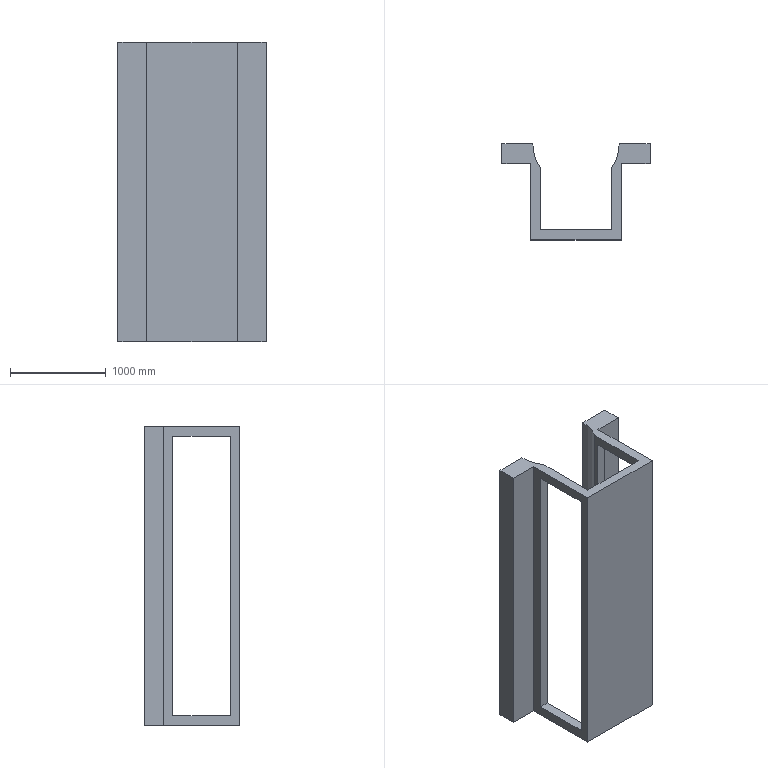Part | SolidWorks | features ICE 10, Extrusion 1, MirrorPattern 1 | 1 solid | 53 faces | box 1550 x 1000 x 3127 mm | volume 797777759 mm3 | plane 39 | cylinder 14 | commonest cylinder face diameters 17 x12 902 x2